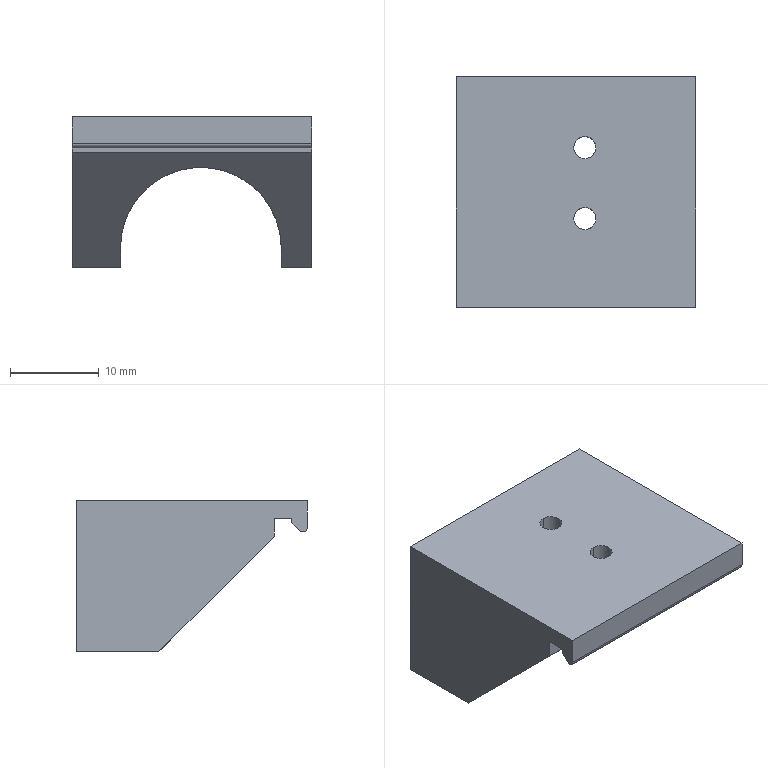CAM job | NX | 3-axis milling, drilling | part box 27 x 26 x 17 mm | stock box 31 x 30 x 18 mm
Tools:
number,name,description,diameter,corner_radius,flute_length,length,flutes
9,D10JING,Milling Tool-5 Parameters,10.0,0.0,50.0,75.0,2
7,D6A45,Milling Tool-5 Parameters,6.0,0.0,50.0,75.0,2
8,2.5ZT,Drilling Tool,2.5,0.0,35.0,50.0,2
10,D10,Milling Tool-5 Parameters,10.0,0.0,50.0,75.0,2
6,D6,Milling Tool-5 Parameters,6.0,0.0,50.0,75.0,2
3,R2,Milling Tool-5 Parameters,4.0,2.0,50.0,75.0,2
2,D2,Milling Tool-5 Parameters,2.0,0.0,50.0,75.0,2
5,D2R0.5,Milling Tool-5 Parameters,2.0,0.5,50.0,75.0,2
Operations:
program,operation,operation_type,tool,method,geometry_group,spindle_rpm,surface_speed,feed_per_tooth,feed_cut,feed_plunge,cut_length_mm,path_length_mm,cut_time_min,machine_time_min
1,FLOOR_WALL,VolumeBased25DMillingOperation,D10JING,METHOD,A,9500.0,298.0,0.0658,1250.0,100.0,324.997,378.997,0.26,0.2654
1,DRILLING,Operation,D6A45,METHOD,A,5000.0,94.0,0.025,250.0,0.0,8.0,87.544,0.032,0.04
1,DRILLING_COPY_COPY_COPY_COPY,Operation,2.5ZT,METHOD,A,2000.0,20.0,0.0375,150.0,0.0,44.502,160.548,0.2967,0.3083
1,ZLEVEL_PROFILE,ZLevelMilling,D10,METHOD,A,9500.0,298.0,0.1316,2500.0,1000.0,4761.652,4835.502,1.927,1.935
1,CAVITY_MILL,CavityMilling,D10,METHOD,A,9500.0,298.0,0.1579,3000.0,1000.0,5093.915,5666.292,1.973,2.03
1,CAVITY_MILL_COPY,CavityMilling,D6,METHOD,A,9509.0,179.0,0.0789,1500.0,1000.0,203.926,659.907,0.1498,0.1954
1,CAVITY_MILL_COPY_COPY,CavityMilling,D2,METHOD,A,9974.0,94.0,0.0501,1000.0,1000.0,547.744,877.464,0.5477,0.5807
1,PLANAR_PROFILE,PlanarMilling,D2,METHOD,A,9500.0,59.0,0.0658,1250.0,100.0,697.0,781.0,0.5576,0.566
1,FIXED_CONTOUR,SurfaceContour,R2,METHOD,A,9500.0,179.0,0.1579,3000.0,1000.0,9426.728,9487.528,3.145,3.151
1,ZLEVEL_PROFILE_1,ZLevelMilling,D2R0.5,METHOD,A,9500.0,89.0,0.1316,2500.0,1000.0,4465.68,4617.869,1.79,1.806
1,ZLEVEL_PROFILE_1_COPY,ZLevelMilling,D2R0.5,METHOD,A,9500.0,89.0,0.1316,2500.0,1000.0,1830.152,2121.187,0.7384,0.7675
1,PLANAR_MILL_COPY_1,PlanarMilling,D6A45,METHOD,A,9500.0,179.0,0.0658,1250.0,100.0,61.763,211.163,0.0494,0.0644
1,刀补9,ZLevelMilling,D10JING,METHOD,A,9500.0,298.0,0.0632,1200.0,1000.0,146.954,236.654,0.1232,0.1322